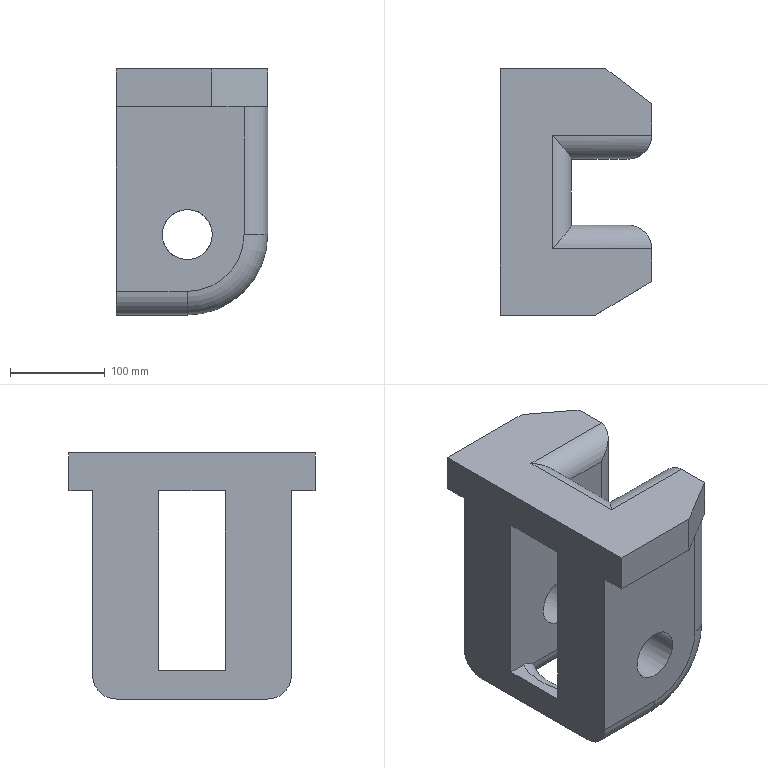Part | NX | features solid 2 | 1 solid | 37 faces | box 160 x 260 x 260 mm | volume 5588314 mm3 | plane 17 | cylinder 15 | torus 5 | commonest cylinder face diameters 50 x10 53 x2 170 x2 40 x1
STEP:
#1=CARTESIAN_POINT('',(710.,440.,280.));
#2=VERTEX_POINT('',#1);
#3=CARTESIAN_POINT('',(765.,440.,280.));
#4=VERTEX_POINT('',#3);
#5=CARTESIAN_POINT('',(710.,440.,280.));
#6=DIRECTION('',(1.,0.,0.));
#7=VECTOR('',#6,1000.);
#8=LINE('',#5,#7);
#9=EDGE_CURVE('',#2,#4,#8,.T.);
#10=ORIENTED_EDGE('',*,*,#9,.T.);
#11=CARTESIAN_POINT('',(784.365,440.,295.));
#12=VERTEX_POINT('',#11);
#13=CARTESIAN_POINT('',(765.,440.,300.));
#14=DIRECTION('',(0.,1.,0.));
#15=DIRECTION('',(0.,0.,-1.));
#16=AXIS2_PLACEMENT_3D('',#13,#14,#15);
#17=CIRCLE('',#16,20.);
#18=EDGE_CURVE('',#4,#12,#17,.F.);
#19=ORIENTED_EDGE('',*,*,#18,.T.);
#20=CARTESIAN_POINT('',(845.,440.,295.));
#21=VERTEX_POINT('',#20);
#22=CARTESIAN_POINT('',(710.,440.,295.));
#23=DIRECTION('',(1.,0.,0.));
#24=VECTOR('',#23,1000.);
#25=LINE('',#22,#24);
#26=EDGE_CURVE('',#21,#12,#25,.F.);
#27=ORIENTED_EDGE('',*,*,#26,.F.);
#28=CARTESIAN_POINT('',(845.,440.,145.));
#29=VERTEX_POINT('',#28);
#30=CARTESIAN_POINT('',(845.,440.,35.));
#31=DIRECTION('',(0.,0.,-1.));
#32=VECTOR('',#31,1000.);
#33=LINE('',#30,#32);
#34=EDGE_CURVE('',#29,#21,#33,.F.);
#35=ORIENTED_EDGE('',*,*,#34,.F.);
#36=CARTESIAN_POINT('',(785.,440.,85.));
#37=VERTEX_POINT('',#36);
#38=CARTESIAN_POINT('',(785.,440.,145.));
#39=DIRECTION('',(0.,-1.,0.));
#40=DIRECTION('',(0.,0.,1.));
#41=AXIS2_PLACEMENT_3D('',#38,#39,#40);
#42=CIRCLE('',#41,60.);
#43=EDGE_CURVE('',#37,#29,#42,.T.);
#44=ORIENTED_EDGE('',*,*,#43,.F.);
#45=CARTESIAN_POINT('',(741.634,440.,85.));
#46=VERTEX_POINT('',#45);
#47=CARTESIAN_POINT('',(710.,440.,85.));
#48=DIRECTION('',(-1.,0.,0.));
#49=VECTOR('',#48,1000.);
#50=LINE('',#47,#49);
#51=EDGE_CURVE('',#46,#37,#50,.F.);
#52=ORIENTED_EDGE('',*,*,#51,.F.);
#53=CARTESIAN_POINT('',(728.668,440.,90.));
#54=VERTEX_POINT('',#53);
#55=CARTESIAN_POINT('',(728.668,440.,90.));
#56=CARTESIAN_POINT('',(733.411,440.,90.));
#57=CARTESIAN_POINT('',(738.187,440.,88.222));
#58=CARTESIAN_POINT('',(741.634,440.,85.));
#59=B_SPLINE_CURVE_WITH_KNOTS('',3,(#55,#56,#57,#58),.UNSPECIFIED.,.F.,.F.,(4,4),(0.08783,0.102),.UNSPECIFIED.);
#60=EDGE_CURVE('',#54,#46,#59,.T.);
#61=ORIENTED_EDGE('',*,*,#60,.F.);
#62=CARTESIAN_POINT('',(710.,440.,90.));
#63=VERTEX_POINT('',#62);
#64=CARTESIAN_POINT('',(710.,440.,90.));
#65=DIRECTION('',(-1.,0.,0.));
#66=VECTOR('',#65,1000.);
#67=LINE('',#64,#66);
#68=EDGE_CURVE('',#54,#63,#67,.T.);
#69=ORIENTED_EDGE('',*,*,#68,.T.);
#70=CARTESIAN_POINT('',(710.,440.,270.));
#71=DIRECTION('',(0.,0.,-1.));
#72=VECTOR('',#71,1000.);
#73=LINE('',#70,#72);
#74=EDGE_CURVE('',#2,#63,#73,.T.);
#75=ORIENTED_EDGE('',*,*,#74,.F.);
#76=EDGE_LOOP('',(#10,#19,#27,#35,#44,#52,#61,#69,#75));
#77=FACE_BOUND('',#76,.T.);
#78=CARTESIAN_POINT('',(785.,440.,171.5));
#79=VERTEX_POINT('',#78);
#80=CARTESIAN_POINT('',(785.,440.,145.));
#81=DIRECTION('',(0.,-1.,0.));
#82=DIRECTION('',(0.,0.,1.));
#83=AXIS2_PLACEMENT_3D('',#80,#81,#82);
#84=CIRCLE('',#83,26.5);
#85=EDGE_CURVE('',#79,#79,#84,.F.);
#86=ORIENTED_EDGE('',*,*,#85,.F.);
#87=EDGE_LOOP('',(#86));
#88=FACE_BOUND('',#87,.T.);
#89=CARTESIAN_POINT('',(710.,440.,35.));
#90=DIRECTION('',(0.,1.,0.));
#91=DIRECTION('',(0.,0.,1.));
#92=AXIS2_PLACEMENT_3D('',#89,#90,#91);
#93=PLANE('',#92);
#94=ADVANCED_FACE('',(#77,#88),#93,.T.);
#95=CARTESIAN_POINT('',(750.,535.,60.));
#96=VERTEX_POINT('',#95);
#97=CARTESIAN_POINT('',(750.,415.,60.));
#98=VERTEX_POINT('',#97);
#99=CARTESIAN_POINT('',(795.,475.,60.));
#100=DIRECTION('',(0.,0.,-1.));
#101=DIRECTION('',(0.,-1.,0.));
#102=AXIS2_PLACEMENT_3D('',#99,#100,#101);
#103=CIRCLE('',#102,75.);
#104=EDGE_CURVE('',#96,#98,#103,.F.);
#105=ORIENTED_EDGE('',*,*,#104,.F.);
#106=CARTESIAN_POINT('',(741.634,510.,85.));
#107=VERTEX_POINT('',#106);
#108=CARTESIAN_POINT('',(750.,535.,60.));
#109=CARTESIAN_POINT('',(749.855,531.571,60.));
#110=CARTESIAN_POINT('',(749.883,524.653,61.451));
#111=CARTESIAN_POINT('',(749.735,516.09,67.563));
#112=CARTESIAN_POINT('',(747.852,510.77,76.551));
#113=CARTESIAN_POINT('',(744.179,510.,82.62));
#114=CARTESIAN_POINT('',(741.634,510.,85.));
#115=B_SPLINE_CURVE_WITH_KNOTS('',3,(#108,#109,#110,#111,#112,#113,#114),.UNSPECIFIED.,.F.,.F.,(4,1,1,1,4),(-0.00004428,0.01025,0.02055,0.03084,0.04114),.UNSPECIFIED.);
#116=EDGE_CURVE('',#96,#107,#115,.T.);
#117=ORIENTED_EDGE('',*,*,#116,.T.);
#118=CARTESIAN_POINT('',(728.668,510.,90.));
#119=VERTEX_POINT('',#118);
#120=CARTESIAN_POINT('',(741.634,510.,85.));
#121=CARTESIAN_POINT('',(738.185,510.,88.224));
#122=CARTESIAN_POINT('',(733.403,510.,90.));
#123=CARTESIAN_POINT('',(728.668,510.,90.));
#124=B_SPLINE_CURVE_WITH_KNOTS('',3,(#120,#121,#122,#123),.UNSPECIFIED.,.F.,.F.,(4,4),(0.0024,0.01656),.UNSPECIFIED.);
#125=EDGE_CURVE('',#107,#119,#124,.T.);
#126=ORIENTED_EDGE('',*,*,#125,.T.);
#127=CARTESIAN_POINT('',(795.,475.,90.));
#128=DIRECTION('',(0.,0.,-1.));
#129=DIRECTION('',(0.,-1.,0.));
#130=AXIS2_PLACEMENT_3D('',#127,#128,#129);
#131=CIRCLE('',#130,75.);
#132=EDGE_CURVE('',#54,#119,#131,.T.);
#133=ORIENTED_EDGE('',*,*,#132,.F.);
#134=ORIENTED_EDGE('',*,*,#60,.T.);
#135=CARTESIAN_POINT('',(741.634,440.,85.));
#136=CARTESIAN_POINT('',(744.172,440.,82.627));
#137=CARTESIAN_POINT('',(747.832,439.25,76.604));
#138=CARTESIAN_POINT('',(749.739,433.909,67.556));
#139=CARTESIAN_POINT('',(749.882,425.357,61.456));
#140=CARTESIAN_POINT('',(749.856,418.421,60.));
#141=CARTESIAN_POINT('',(750.,415.,60.));
#142=B_SPLINE_CURVE_WITH_KNOTS('',3,(#135,#136,#137,#138,#139,#140,#141),.UNSPECIFIED.,.F.,.F.,(4,1,1,1,4),(0.000000289,0.01027,0.02055,0.03082,0.04109),.UNSPECIFIED.);
#143=EDGE_CURVE('',#46,#98,#142,.T.);
#144=ORIENTED_EDGE('',*,*,#143,.T.);
#145=EDGE_LOOP('',(#105,#117,#126,#133,#134,#144));
#146=FACE_BOUND('',#145,.T.);
#147=CARTESIAN_POINT('',(795.,475.,75.));
#148=DIRECTION('',(0.,0.,-1.));
#149=DIRECTION('',(0.,-1.,0.));
#150=AXIS2_PLACEMENT_3D('',#147,#148,#149);
#151=TOROIDAL_SURFACE('',#150,75.,15.);
#152=ADVANCED_FACE('',(#146),#151,.T.);
#153=CARTESIAN_POINT('',(710.,555.,60.));
#154=VERTEX_POINT('',#153);
#155=CARTESIAN_POINT('',(710.,395.,60.));
#156=VERTEX_POINT('',#155);
#157=CARTESIAN_POINT('',(710.,455.,60.));
#158=DIRECTION('',(0.,-1.,0.));
#159=VECTOR('',#158,1000.);
#160=LINE('',#157,#159);
#161=EDGE_CURVE('',#154,#156,#160,.T.);
#162=ORIENTED_EDGE('',*,*,#161,.F.);
#163=CARTESIAN_POINT('',(785.,555.,60.));
#164=VERTEX_POINT('',#163);
#165=CARTESIAN_POINT('',(785.,555.,60.));
#166=DIRECTION('',(1.,0.,0.));
#167=VECTOR('',#166,1000.);
#168=LINE('',#165,#167);
#169=EDGE_CURVE('',#164,#154,#168,.F.);
#170=ORIENTED_EDGE('',*,*,#169,.F.);
#171=CARTESIAN_POINT('',(785.,535.,60.));
#172=VERTEX_POINT('',#171);
#173=CARTESIAN_POINT('',(785.,455.,60.));
#174=DIRECTION('',(0.,1.,0.));
#175=VECTOR('',#174,1000.);
#176=LINE('',#173,#175);
#177=EDGE_CURVE('',#172,#164,#176,.T.);
#178=ORIENTED_EDGE('',*,*,#177,.F.);
#179=CARTESIAN_POINT('',(785.,535.,60.));
#180=DIRECTION('',(-1.,0.,0.));
#181=VECTOR('',#180,1000.);
#182=LINE('',#179,#181);
#183=EDGE_CURVE('',#96,#172,#182,.F.);
#184=ORIENTED_EDGE('',*,*,#183,.F.);
#185=ORIENTED_EDGE('',*,*,#104,.T.);
#186=CARTESIAN_POINT('',(785.,415.,60.));
#187=VERTEX_POINT('',#186);
#188=CARTESIAN_POINT('',(785.,415.,60.));
#189=DIRECTION('',(-1.,0.,0.));
#190=VECTOR('',#189,1000.);
#191=LINE('',#188,#190);
#192=EDGE_CURVE('',#187,#98,#191,.T.);
#193=ORIENTED_EDGE('',*,*,#192,.F.);
#194=CARTESIAN_POINT('',(785.,395.,60.));
#195=VERTEX_POINT('',#194);
#196=CARTESIAN_POINT('',(785.,315.,60.));
#197=DIRECTION('',(0.,1.,0.));
#198=VECTOR('',#197,1000.);
#199=LINE('',#196,#198);
#200=EDGE_CURVE('',#195,#187,#199,.T.);
#201=ORIENTED_EDGE('',*,*,#200,.F.);
#202=CARTESIAN_POINT('',(785.,395.,60.));
#203=DIRECTION('',(1.,0.,0.));
#204=VECTOR('',#203,1000.);
#205=LINE('',#202,#204);
#206=EDGE_CURVE('',#156,#195,#205,.T.);
#207=ORIENTED_EDGE('',*,*,#206,.F.);
#208=EDGE_LOOP('',(#162,#170,#178,#184,#185,#193,#201,#207));
#209=FACE_BOUND('',#208,.T.);
#210=CARTESIAN_POINT('',(785.,455.,60.));
#211=DIRECTION('',(0.,0.,-1.));
#212=DIRECTION('',(-1.,0.,0.));
#213=AXIS2_PLACEMENT_3D('',#210,#211,#212);
#214=PLANE('',#213);
#215=ADVANCED_FACE('',(#209),#214,.T.);
#216=CARTESIAN_POINT('',(765.,415.,320.));
#217=VERTEX_POINT('',#216);
#218=CARTESIAN_POINT('',(784.365,440.,295.));
#219=CARTESIAN_POINT('',(784.836,440.,296.824));
#220=CARTESIAN_POINT('',(785.148,439.689,299.624));
#221=CARTESIAN_POINT('',(784.832,438.765,302.842));
#222=CARTESIAN_POINT('',(784.481,438.097,304.604));
#223=CARTESIAN_POINT('',(784.097,437.471,305.986));
#224=CARTESIAN_POINT('',(783.748,436.945,306.992));
#225=CARTESIAN_POINT('',(783.16,436.104,308.447));
#226=CARTESIAN_POINT('',(782.267,434.912,310.182));
#227=CARTESIAN_POINT('',(781.153,433.51,311.844));
#228=CARTESIAN_POINT('',(780.247,432.405,312.954));
#229=CARTESIAN_POINT('',(779.714,431.764,313.551));
#230=CARTESIAN_POINT('',(779.249,431.207,314.038));
#231=CARTESIAN_POINT('',(778.959,430.862,314.325));
#232=CARTESIAN_POINT('',(778.49,430.306,314.772));
#233=CARTESIAN_POINT('',(777.656,429.324,315.509));
#234=CARTESIAN_POINT('',(776.589,428.081,316.326));
#235=CARTESIAN_POINT('',(775.424,426.742,317.08));
#236=CARTESIAN_POINT('',(774.497,425.682,317.612));
#237=CARTESIAN_POINT('',(773.688,424.763,318.021));
#238=CARTESIAN_POINT('',(773.089,424.083,318.293));
#239=CARTESIAN_POINT('',(772.758,423.709,318.435));
#240=CARTESIAN_POINT('',(772.456,423.367,318.559));
#241=CARTESIAN_POINT('',(772.346,423.243,318.602));
#242=CARTESIAN_POINT('',(772.124,422.991,318.689));
#243=CARTESIAN_POINT('',(771.748,422.566,318.83));
#244=CARTESIAN_POINT('',(771.144,421.881,319.039));
#245=CARTESIAN_POINT('',(770.34,420.973,319.281));
#246=CARTESIAN_POINT('',(769.15,419.635,319.582));
#247=CARTESIAN_POINT('',(767.445,417.727,319.892));
#248=CARTESIAN_POINT('',(765.851,415.951,320.));
#249=CARTESIAN_POINT('',(765.,415.,320.));
#250=B_SPLINE_CURVE_WITH_KNOTS('',3,(#218,#219,#220,#221,#222,#223,#224,#225,#226,#227,#228,#229,#230,#231,#232,#233,#234,#235,#236,#237,#238,#239,#240,#241,#242,#243,#244,#245,#246,#247,#248,#249),.UNSPECIFIED.,.F.,.F.,(4,1,1,1,1,1,1,1,1,1,1,1,1,1,1,1,1,1,1,1,1,1,1,1,1,1,1,1,1,4),(0.,0.125,0.1875,0.2188,0.25,0.2812,0.3125,0.375,0.4375,0.4688,0.4844,0.5,0.5156,0.5312,0.5625,0.625,0.6562,0.6875,0.7188,0.7344,0.7422,0.75,0.7578,0.7656,0.7812,0.8125,0.8438,0.875,0.9375,1.),.UNSPECIFIED.);
#251=EDGE_CURVE('',#12,#217,#250,.T.);
#252=ORIENTED_EDGE('',*,*,#251,.F.);
#253=ORIENTED_EDGE('',*,*,#18,.F.);
#254=CARTESIAN_POINT('',(765.,510.,280.));
#255=VERTEX_POINT('',#254);
#256=CARTESIAN_POINT('',(765.,400.,280.));
#257=DIRECTION('',(0.,1.,0.));
#258=VECTOR('',#257,1000.);
#259=LINE('',#256,#258);
#260=EDGE_CURVE('',#255,#4,#259,.F.);
#261=ORIENTED_EDGE('',*,*,#260,.F.);
#262=CARTESIAN_POINT('',(784.365,510.,295.));
#263=VERTEX_POINT('',#262);
#264=CARTESIAN_POINT('',(765.,510.,300.));
#265=DIRECTION('',(0.,1.,0.));
#266=DIRECTION('',(0.,0.,-1.));
#267=AXIS2_PLACEMENT_3D('',#264,#265,#266);
#268=CIRCLE('',#267,20.);
#269=EDGE_CURVE('',#263,#255,#268,.T.);
#270=ORIENTED_EDGE('',*,*,#269,.F.);
#271=CARTESIAN_POINT('',(765.,535.,320.));
#272=VERTEX_POINT('',#271);
#273=CARTESIAN_POINT('',(784.365,510.,295.));
#274=CARTESIAN_POINT('',(784.836,510.,296.824));
#275=CARTESIAN_POINT('',(785.148,510.311,299.624));
#276=CARTESIAN_POINT('',(784.832,511.235,302.842));
#277=CARTESIAN_POINT('',(784.481,511.903,304.604));
#278=CARTESIAN_POINT('',(784.097,512.529,305.986));
#279=CARTESIAN_POINT('',(783.748,513.055,306.992));
#280=CARTESIAN_POINT('',(783.16,513.896,308.447));
#281=CARTESIAN_POINT('',(782.267,515.088,310.182));
#282=CARTESIAN_POINT('',(781.153,516.49,311.844));
#283=CARTESIAN_POINT('',(780.247,517.595,312.954));
#284=CARTESIAN_POINT('',(779.714,518.236,313.551));
#285=CARTESIAN_POINT('',(779.249,518.793,314.038));
#286=CARTESIAN_POINT('',(778.959,519.138,314.325));
#287=CARTESIAN_POINT('',(778.49,519.694,314.772));
#288=CARTESIAN_POINT('',(777.656,520.676,315.509));
#289=CARTESIAN_POINT('',(776.589,521.919,316.326));
#290=CARTESIAN_POINT('',(775.424,523.258,317.08));
#291=CARTESIAN_POINT('',(774.497,524.318,317.612));
#292=CARTESIAN_POINT('',(773.688,525.237,318.021));
#293=CARTESIAN_POINT('',(773.089,525.917,318.293));
#294=CARTESIAN_POINT('',(772.758,526.291,318.435));
#295=CARTESIAN_POINT('',(772.456,526.633,318.559));
#296=CARTESIAN_POINT('',(772.346,526.757,318.602));
#297=CARTESIAN_POINT('',(772.124,527.009,318.689));
#298=CARTESIAN_POINT('',(771.748,527.434,318.83));
#299=CARTESIAN_POINT('',(771.144,528.119,319.039));
#300=CARTESIAN_POINT('',(770.34,529.027,319.281));
#301=CARTESIAN_POINT('',(769.15,530.365,319.582));
#302=CARTESIAN_POINT('',(767.445,532.273,319.892));
#303=CARTESIAN_POINT('',(765.851,534.049,320.));
#304=CARTESIAN_POINT('',(765.,535.,320.));
#305=B_SPLINE_CURVE_WITH_KNOTS('',3,(#273,#274,#275,#276,#277,#278,#279,#280,#281,#282,#283,#284,#285,#286,#287,#288,#289,#290,#291,#292,#293,#294,#295,#296,#297,#298,#299,#300,#301,#302,#303,#304),.UNSPECIFIED.,.F.,.F.,(4,1,1,1,1,1,1,1,1,1,1,1,1,1,1,1,1,1,1,1,1,1,1,1,1,1,1,1,1,4),(0.,0.125,0.1875,0.2188,0.25,0.2812,0.3125,0.375,0.4375,0.4688,0.4844,0.5,0.5156,0.5312,0.5625,0.625,0.6562,0.6875,0.7188,0.7344,0.7422,0.75,0.7578,0.7656,0.7812,0.8125,0.8438,0.875,0.9375,1.),.UNSPECIFIED.);
#306=EDGE_CURVE('',#263,#272,#305,.T.);
#307=ORIENTED_EDGE('',*,*,#306,.T.);
#308=CARTESIAN_POINT('',(765.,510.,320.));
#309=DIRECTION('',(0.,1.,0.));
#310=VECTOR('',#309,1000.);
#311=LINE('',#308,#310);
#312=EDGE_CURVE('',#217,#272,#311,.T.);
#313=ORIENTED_EDGE('',*,*,#312,.F.);
#314=EDGE_LOOP('',(#252,#253,#261,#270,#307,#313));
#315=FACE_BOUND('',#314,.T.);
#316=CARTESIAN_POINT('',(765.,510.,300.));
#317=DIRECTION('',(0.,-1.,0.));
#318=DIRECTION('',(0.,0.,1.));
#319=AXIS2_PLACEMENT_3D('',#316,#317,#318);
#320=CYLINDRICAL_SURFACE('',#319,20.);
#321=ADVANCED_FACE('',(#315),#320,.T.);
#322=ORIENTED_EDGE('',*,*,#312,.T.);
#323=CARTESIAN_POINT('',(870.,535.,320.));
#324=VERTEX_POINT('',#323);
#325=CARTESIAN_POINT('',(765.,535.,320.));
#326=DIRECTION('',(1.,0.,0.));
#327=VECTOR('',#326,1000.);
#328=LINE('',#325,#327);
#329=EDGE_CURVE('',#324,#272,#328,.F.);
#330=ORIENTED_EDGE('',*,*,#329,.F.);
#331=CARTESIAN_POINT('',(870.,568.232,320.));
#332=VERTEX_POINT('',#331);
#333=CARTESIAN_POINT('',(870.,455.,320.));
#334=DIRECTION('',(0.,-1.,0.));
#335=VECTOR('',#334,1000.);
#336=LINE('',#333,#335);
#337=EDGE_CURVE('',#332,#324,#336,.T.);
#338=ORIENTED_EDGE('',*,*,#337,.F.);
#339=CARTESIAN_POINT('',(821.621,605.,320.));
#340=VERTEX_POINT('',#339);
#341=CARTESIAN_POINT('',(938.114,516.465,320.));
#342=DIRECTION('',(0.7962,-0.6051,0.));
#343=VECTOR('',#342,1000.);
#344=LINE('',#341,#343);
#345=EDGE_CURVE('',#332,#340,#344,.F.);
#346=ORIENTED_EDGE('',*,*,#345,.T.);
#347=CARTESIAN_POINT('',(710.,605.,320.));
#348=VERTEX_POINT('',#347);
#349=CARTESIAN_POINT('',(10.,605.,320.));
#350=DIRECTION('',(1.,0.,0.));
#351=VECTOR('',#350,1000.);
#352=LINE('',#349,#351);
#353=EDGE_CURVE('',#340,#348,#352,.F.);
#354=ORIENTED_EDGE('',*,*,#353,.T.);
#355=CARTESIAN_POINT('',(710.,345.,320.));
#356=VERTEX_POINT('',#355);
#357=CARTESIAN_POINT('',(710.,510.,320.));
#358=DIRECTION('',(0.,1.,0.));
#359=VECTOR('',#358,1000.);
#360=LINE('',#357,#359);
#361=EDGE_CURVE('',#348,#356,#360,.F.);
#362=ORIENTED_EDGE('',*,*,#361,.T.);
#363=CARTESIAN_POINT('',(810.84,345.,320.));
#364=VERTEX_POINT('',#363);
#365=CARTESIAN_POINT('',(785.,345.,320.));
#366=DIRECTION('',(-1.,0.,0.));
#367=VECTOR('',#366,1000.);
#368=LINE('',#365,#367);
#369=EDGE_CURVE('',#364,#356,#368,.T.);
#370=ORIENTED_EDGE('',*,*,#369,.F.);
#371=CARTESIAN_POINT('',(870.,380.496,320.));
#372=VERTEX_POINT('',#371);
#373=CARTESIAN_POINT('',(778.605,325.659,320.));
#374=DIRECTION('',(0.8575,0.5145,0.));
#375=VECTOR('',#374,1000.);
#376=LINE('',#373,#375);
#377=EDGE_CURVE('',#364,#372,#376,.T.);
#378=ORIENTED_EDGE('',*,*,#377,.T.);
#379=CARTESIAN_POINT('',(870.,415.,320.));
#380=VERTEX_POINT('',#379);
#381=CARTESIAN_POINT('',(870.,315.,320.));
#382=DIRECTION('',(0.,-1.,0.));
#383=VECTOR('',#382,1000.);
#384=LINE('',#381,#383);
#385=EDGE_CURVE('',#380,#372,#384,.T.);
#386=ORIENTED_EDGE('',*,*,#385,.F.);
#387=CARTESIAN_POINT('',(785.,415.,320.));
#388=DIRECTION('',(1.,0.,0.));
#389=VECTOR('',#388,1000.);
#390=LINE('',#387,#389);
#391=EDGE_CURVE('',#217,#380,#390,.T.);
#392=ORIENTED_EDGE('',*,*,#391,.F.);
#393=EDGE_LOOP('',(#322,#330,#338,#346,#354,#362,#370,#378,#386,#392));
#394=FACE_BOUND('',#393,.T.);
#395=CARTESIAN_POINT('',(710.,510.,320.));
#396=DIRECTION('',(0.,0.,-1.));
#397=DIRECTION('',(0.,1.,0.));
#398=AXIS2_PLACEMENT_3D('',#395,#396,#397);
#399=PLANE('',#398);
#400=ADVANCED_FACE('',(#394),#399,.F.);
#401=CARTESIAN_POINT('',(710.,510.,90.));
#402=VERTEX_POINT('',#401);
#403=CARTESIAN_POINT('',(710.,510.,280.));
#404=VERTEX_POINT('',#403);
#405=CARTESIAN_POINT('',(710.,510.,60.));
#406=DIRECTION('',(0.,0.,1.));
#407=VECTOR('',#406,1000.);
#408=LINE('',#405,#407);
#409=EDGE_CURVE('',#402,#404,#408,.T.);
#410=ORIENTED_EDGE('',*,*,#409,.T.);
#411=CARTESIAN_POINT('',(710.,510.,280.));
#412=DIRECTION('',(0.,1.,0.));
#413=VECTOR('',#412,1000.);
#414=LINE('',#411,#413);
#415=EDGE_CURVE('',#404,#2,#414,.F.);
#416=ORIENTED_EDGE('',*,*,#415,.T.);
#417=ORIENTED_EDGE('',*,*,#74,.T.);
#418=CARTESIAN_POINT('',(710.,510.,90.));
#419=DIRECTION('',(0.,-1.,0.));
#420=VECTOR('',#419,1000.);
#421=LINE('',#418,#420);
#422=EDGE_CURVE('',#402,#63,#421,.T.);
#423=ORIENTED_EDGE('',*,*,#422,.F.);
#424=EDGE_LOOP('',(#410,#416,#417,#423));
#425=FACE_BOUND('',#424,.T.);
#426=ORIENTED_EDGE('',*,*,#361,.F.);
#427=CARTESIAN_POINT('',(710.,605.,280.));
#428=VERTEX_POINT('',#427);
#429=CARTESIAN_POINT('',(710.,605.,155.));
#430=DIRECTION('',(0.,0.,1.));
#431=VECTOR('',#430,1000.);
#432=LINE('',#429,#431);
#433=EDGE_CURVE('',#348,#428,#432,.F.);
#434=ORIENTED_EDGE('',*,*,#433,.T.);
#435=CARTESIAN_POINT('',(710.,580.,280.));
#436=VERTEX_POINT('',#435);
#437=CARTESIAN_POINT('',(710.,620.,280.));
#438=DIRECTION('',(0.,-1.,0.));
#439=VECTOR('',#438,1000.);
#440=LINE('',#437,#439);
#441=EDGE_CURVE('',#428,#436,#440,.T.);
#442=ORIENTED_EDGE('',*,*,#441,.T.);
#443=CARTESIAN_POINT('',(710.,580.,85.));
#444=VERTEX_POINT('',#443);
#445=CARTESIAN_POINT('',(710.,580.,95.));
#446=DIRECTION('',(0.,0.,-1.));
#447=VECTOR('',#446,1000.);
#448=LINE('',#445,#447);
#449=EDGE_CURVE('',#436,#444,#448,.T.);
#450=ORIENTED_EDGE('',*,*,#449,.T.);
#451=CARTESIAN_POINT('',(710.,555.,85.));
#452=DIRECTION('',(1.,0.,0.));
#453=DIRECTION('',(0.,0.,-1.));
#454=AXIS2_PLACEMENT_3D('',#451,#452,#453);
#455=CIRCLE('',#454,25.);
#456=EDGE_CURVE('',#154,#444,#455,.T.);
#457=ORIENTED_EDGE('',*,*,#456,.F.);
#458=ORIENTED_EDGE('',*,*,#161,.T.);
#459=CARTESIAN_POINT('',(710.,370.,85.));
#460=VERTEX_POINT('',#459);
#461=CARTESIAN_POINT('',(710.,395.,85.));
#462=DIRECTION('',(1.,0.,0.));
#463=DIRECTION('',(0.,0.,-1.));
#464=AXIS2_PLACEMENT_3D('',#461,#462,#463);
#465=CIRCLE('',#464,25.);
#466=EDGE_CURVE('',#460,#156,#465,.T.);
#467=ORIENTED_EDGE('',*,*,#466,.F.);
#468=CARTESIAN_POINT('',(710.,370.,280.));
#469=VERTEX_POINT('',#468);
#470=CARTESIAN_POINT('',(710.,370.,70.));
#471=DIRECTION('',(0.,0.,1.));
#472=VECTOR('',#471,1000.);
#473=LINE('',#470,#472);
#474=EDGE_CURVE('',#460,#469,#473,.T.);
#475=ORIENTED_EDGE('',*,*,#474,.T.);
#476=CARTESIAN_POINT('',(710.,345.,280.));
#477=VERTEX_POINT('',#476);
#478=CARTESIAN_POINT('',(710.,285.,280.));
#479=DIRECTION('',(0.,-1.,0.));
#480=VECTOR('',#479,1000.);
#481=LINE('',#478,#480);
#482=EDGE_CURVE('',#469,#477,#481,.T.);
#483=ORIENTED_EDGE('',*,*,#482,.T.);
#484=CARTESIAN_POINT('',(710.,345.,245.));
#485=DIRECTION('',(0.,0.,-1.));
#486=VECTOR('',#485,1000.);
#487=LINE('',#484,#486);
#488=EDGE_CURVE('',#356,#477,#487,.T.);
#489=ORIENTED_EDGE('',*,*,#488,.F.);
#490=EDGE_LOOP('',(#426,#434,#442,#450,#457,#458,#467,#475,#483,#489));
#491=FACE_BOUND('',#490,.T.);
#492=CARTESIAN_POINT('',(710.,340.,270.));
#493=DIRECTION('',(-1.,0.,0.));
#494=DIRECTION('',(0.,-1.,0.));
#495=AXIS2_PLACEMENT_3D('',#492,#493,#494);
#496=PLANE('',#495);
#497=ADVANCED_FACE('',(#425,#491),#496,.T.);
#498=CARTESIAN_POINT('',(845.,370.,145.));
#499=VERTEX_POINT('',#498);
#500=CARTESIAN_POINT('',(870.,395.,145.));
#501=VERTEX_POINT('',#500);
#502=CARTESIAN_POINT('',(845.,395.,145.));
#503=DIRECTION('',(0.,0.,1.));
#504=DIRECTION('',(0.,1.,0.));
#505=AXIS2_PLACEMENT_3D('',#502,#503,#504);
#506=CIRCLE('',#505,25.);
#507=EDGE_CURVE('',#499,#501,#506,.T.);
#508=ORIENTED_EDGE('',*,*,#507,.F.);
#509=CARTESIAN_POINT('',(785.,370.,85.));
#510=VERTEX_POINT('',#509);
#511=CARTESIAN_POINT('',(785.,370.,145.));
#512=DIRECTION('',(0.,1.,0.));
#513=DIRECTION('',(0.,0.,-1.));
#514=AXIS2_PLACEMENT_3D('',#511,#512,#513);
#515=CIRCLE('',#514,60.);
#516=EDGE_CURVE('',#499,#510,#515,.T.);
#517=ORIENTED_EDGE('',*,*,#516,.T.);
#518=CARTESIAN_POINT('',(785.,395.,85.));
#519=DIRECTION('',(1.,0.,0.));
#520=DIRECTION('',(0.,0.,-1.));
#521=AXIS2_PLACEMENT_3D('',#518,#519,#520);
#522=CIRCLE('',#521,25.);
#523=EDGE_CURVE('',#510,#195,#522,.T.);
#524=ORIENTED_EDGE('',*,*,#523,.T.);
#525=CARTESIAN_POINT('',(785.,395.,145.));
#526=DIRECTION('',(0.,1.,0.));
#527=DIRECTION('',(0.,0.,-1.));
#528=AXIS2_PLACEMENT_3D('',#525,#526,#527);
#529=CIRCLE('',#528,85.);
#530=EDGE_CURVE('',#195,#501,#529,.F.);
#531=ORIENTED_EDGE('',*,*,#530,.T.);
#532=EDGE_LOOP('',(#508,#517,#524,#531));
#533=FACE_BOUND('',#532,.T.);
#534=CARTESIAN_POINT('',(785.,395.,145.));
#535=DIRECTION('',(0.,-1.,0.));
#536=DIRECTION('',(0.,0.,-1.));
#537=AXIS2_PLACEMENT_3D('',#534,#535,#536);
#538=TOROIDAL_SURFACE('',#537,60.,25.);
#539=ADVANCED_FACE('',(#533),#538,.T.);
#540=CARTESIAN_POINT('',(870.,395.,280.));
#541=VERTEX_POINT('',#540);
#542=CARTESIAN_POINT('',(870.,395.,70.));
#543=DIRECTION('',(0.,0.,-1.));
#544=VECTOR('',#543,1000.);
#545=LINE('',#542,#544);
#546=EDGE_CURVE('',#501,#541,#545,.F.);
#547=ORIENTED_EDGE('',*,*,#546,.T.);
#548=CARTESIAN_POINT('',(845.,370.,280.));
#549=VERTEX_POINT('',#548);
#550=CARTESIAN_POINT('',(845.,395.,280.));
#551=DIRECTION('',(0.,0.,1.));
#552=DIRECTION('',(0.,1.,0.));
#553=AXIS2_PLACEMENT_3D('',#550,#551,#552);
#554=CIRCLE('',#553,25.);
#555=EDGE_CURVE('',#541,#549,#554,.F.);
#556=ORIENTED_EDGE('',*,*,#555,.T.);
#557=CARTESIAN_POINT('',(845.,370.,70.));
#558=DIRECTION('',(0.,0.,-1.));
#559=VECTOR('',#558,1000.);
#560=LINE('',#557,#559);
#561=EDGE_CURVE('',#549,#499,#560,.T.);
#562=ORIENTED_EDGE('',*,*,#561,.T.);
#563=ORIENTED_EDGE('',*,*,#507,.T.);
#564=EDGE_LOOP('',(#547,#556,#562,#563));
#565=FACE_BOUND('',#564,.T.);
#566=CARTESIAN_POINT('',(845.,395.,70.));
#567=DIRECTION('',(0.,0.,-1.));
#568=DIRECTION('',(0.,1.,0.));
#569=AXIS2_PLACEMENT_3D('',#566,#567,#568);
#570=CYLINDRICAL_SURFACE('',#569,25.);
#571=ADVANCED_FACE('',(#565),#570,.T.);
#572=CARTESIAN_POINT('',(870.,415.,145.));
#573=VERTEX_POINT('',#572);
#574=CARTESIAN_POINT('',(845.,415.,145.));
#575=DIRECTION('',(0.,0.,1.));
#576=DIRECTION('',(0.,1.,0.));
#577=AXIS2_PLACEMENT_3D('',#574,#575,#576);
#578=CIRCLE('',#577,25.);
#579=EDGE_CURVE('',#573,#29,#578,.T.);
#580=ORIENTED_EDGE('',*,*,#579,.F.);
#581=CARTESIAN_POINT('',(785.,415.,145.));
#582=DIRECTION('',(0.,-1.,0.));
#583=DIRECTION('',(0.,0.,1.));
#584=AXIS2_PLACEMENT_3D('',#581,#582,#583);
#585=CIRCLE('',#584,85.);
#586=EDGE_CURVE('',#573,#187,#585,.F.);
#587=ORIENTED_EDGE('',*,*,#586,.T.);
#588=CARTESIAN_POINT('',(785.,415.,85.));
#589=DIRECTION('',(1.,0.,0.));
#590=DIRECTION('',(0.,0.,-1.));
#591=AXIS2_PLACEMENT_3D('',#588,#589,#590);
#592=CIRCLE('',#591,25.);
#593=EDGE_CURVE('',#187,#37,#592,.T.);
#594=ORIENTED_EDGE('',*,*,#593,.T.);
#595=ORIENTED_EDGE('',*,*,#43,.T.);
#596=EDGE_LOOP('',(#580,#587,#594,#595));
#597=FACE_BOUND('',#596,.T.);
#598=CARTESIAN_POINT('',(785.,415.,145.));
#599=DIRECTION('',(0.,1.,0.));
#600=DIRECTION('',(0.,0.,1.));
#601=AXIS2_PLACEMENT_3D('',#598,#599,#600);
#602=TOROIDAL_SURFACE('',#601,60.,25.);
#603=ADVANCED_FACE('',(#597),#602,.T.);
#604=ORIENTED_EDGE('',*,*,#34,.T.);
#605=CARTESIAN_POINT('',(845.,415.,295.));
#606=DIRECTION('',(-0.7071,0.,0.7071));
#607=DIRECTION('',(0.7071,0.,0.7071));
#608=AXIS2_PLACEMENT_3D('',#605,#606,#607);
#609=ELLIPSE('',#608,35.355,25.);
#610=EDGE_CURVE('',#380,#21,#609,.T.);
#611=ORIENTED_EDGE('',*,*,#610,.F.);
#612=CARTESIAN_POINT('',(870.,415.,70.));
#613=DIRECTION('',(0.,0.,-1.));
#614=VECTOR('',#613,1000.);
#615=LINE('',#612,#614);
#616=EDGE_CURVE('',#380,#573,#615,.T.);
#617=ORIENTED_EDGE('',*,*,#616,.T.);
#618=ORIENTED_EDGE('',*,*,#579,.T.);
#619=EDGE_LOOP('',(#604,#611,#617,#618));
#620=FACE_BOUND('',#619,.T.);
#621=CARTESIAN_POINT('',(845.,415.,70.));
#622=DIRECTION('',(0.,0.,-1.));
#623=DIRECTION('',(0.,1.,0.));
#624=AXIS2_PLACEMENT_3D('',#621,#622,#623);
#625=CYLINDRICAL_SURFACE('',#624,25.);
#626=ADVANCED_FACE('',(#620),#625,.T.);
#627=CARTESIAN_POINT('',(811.5,370.,145.));
#628=VERTEX_POINT('',#627);
#629=CARTESIAN_POINT('',(785.,370.,145.));
#630=DIRECTION('',(0.,1.,0.));
#631=DIRECTION('',(1.,0.,0.));
#632=AXIS2_PLACEMENT_3D('',#629,#630,#631);
#633=CIRCLE('',#632,26.5);
#634=EDGE_CURVE('',#628,#628,#633,.T.);
#635=ORIENTED_EDGE('',*,*,#634,.F.);
#636=EDGE_LOOP('',(#635));
#637=FACE_BOUND('',#636,.T.);
#638=ORIENTED_EDGE('',*,*,#85,.T.);
#639=EDGE_LOOP('',(#638));
#640=FACE_BOUND('',#639,.T.);
#641=CARTESIAN_POINT('',(785.,185.,145.));
#642=DIRECTION('',(0.,1.,0.));
#643=DIRECTION('',(-1.,0.,0.));
#644=AXIS2_PLACEMENT_3D('',#641,#642,#643);
#645=CYLINDRICAL_SURFACE('',#644,26.5);
#646=ADVANCED_FACE('',(#637,#640),#645,.F.);
#647=ORIENTED_EDGE('',*,*,#482,.F.);
#648=CARTESIAN_POINT('',(870.,370.,280.));
#649=DIRECTION('',(-1.,0.,0.));
#650=VECTOR('',#649,1000.);
#651=LINE('',#648,#650);
#652=EDGE_CURVE('',#549,#469,#651,.T.);
#653=ORIENTED_EDGE('',*,*,#652,.F.);
#654=ORIENTED_EDGE('',*,*,#555,.F.);
#655=CARTESIAN_POINT('',(870.,380.496,280.));
#656=VERTEX_POINT('',#655);
#657=CARTESIAN_POINT('',(870.,370.,280.));
#658=DIRECTION('',(0.,-1.,0.));
#659=VECTOR('',#658,1000.);
#660=LINE('',#657,#659);
#661=EDGE_CURVE('',#541,#656,#660,.T.);
#662=ORIENTED_EDGE('',*,*,#661,.T.);
#663=CARTESIAN_POINT('',(810.84,345.,280.));
#664=VERTEX_POINT('',#663);
#665=CARTESIAN_POINT('',(865.37,377.717,280.));
#666=DIRECTION('',(-0.8575,-0.5145,0.));
#667=VECTOR('',#666,1000.);
#668=LINE('',#665,#667);
#669=EDGE_CURVE('',#656,#664,#668,.T.);
#670=ORIENTED_EDGE('',*,*,#669,.T.);
#671=CARTESIAN_POINT('',(700.,345.,280.));
#672=DIRECTION('',(1.,0.,0.));
#673=VECTOR('',#672,1000.);
#674=LINE('',#671,#673);
#675=EDGE_CURVE('',#477,#664,#674,.T.);
#676=ORIENTED_EDGE('',*,*,#675,.F.);
#677=EDGE_LOOP('',(#647,#653,#654,#662,#670,#676));
#678=FACE_BOUND('',#677,.T.);
#679=CARTESIAN_POINT('',(700.,285.,280.));
#680=DIRECTION('',(0.,0.,-1.));
#681=DIRECTION('',(0.,-1.,0.));
#682=AXIS2_PLACEMENT_3D('',#679,#680,#681);
#683=PLANE('',#682);
#684=ADVANCED_FACE('',(#678),#683,.T.);
#685=ORIENTED_EDGE('',*,*,#516,.F.);
#686=ORIENTED_EDGE('',*,*,#561,.F.);
#687=ORIENTED_EDGE('',*,*,#652,.T.);
#688=ORIENTED_EDGE('',*,*,#474,.F.);
#689=CARTESIAN_POINT('',(785.,370.,85.));
#690=DIRECTION('',(1.,0.,0.));
#691=VECTOR('',#690,1000.);
#692=LINE('',#689,#691);
#693=EDGE_CURVE('',#510,#460,#692,.F.);
#694=ORIENTED_EDGE('',*,*,#693,.F.);
#695=EDGE_LOOP('',(#685,#686,#687,#688,#694));
#696=FACE_BOUND('',#695,.T.);
#697=ORIENTED_EDGE('',*,*,#634,.T.);
#698=EDGE_LOOP('',(#697));
#699=FACE_BOUND('',#698,.T.);
#700=CARTESIAN_POINT('',(785.,370.,70.));
#701=DIRECTION('',(0.,-1.,0.));
#702=DIRECTION('',(1.,0.,0.));
#703=AXIS2_PLACEMENT_3D('',#700,#701,#702);
#704=PLANE('',#703);
#705=ADVANCED_FACE('',(#696,#699),#704,.T.);
#706=ORIENTED_EDGE('',*,*,#466,.T.);
#707=ORIENTED_EDGE('',*,*,#206,.T.);
#708=ORIENTED_EDGE('',*,*,#523,.F.);
#709=ORIENTED_EDGE('',*,*,#693,.T.);
#710=EDGE_LOOP('',(#706,#707,#708,#709));
#711=FACE_BOUND('',#710,.T.);
#712=CARTESIAN_POINT('',(785.,395.,85.));
#713=DIRECTION('',(1.,0.,0.));
#714=DIRECTION('',(0.,0.,1.));
#715=AXIS2_PLACEMENT_3D('',#712,#713,#714);
#716=CYLINDRICAL_SURFACE('',#715,25.);
#717=ADVANCED_FACE('',(#711),#716,.T.);
#718=ORIENTED_EDGE('',*,*,#200,.T.);
#719=ORIENTED_EDGE('',*,*,#586,.F.);
#720=CARTESIAN_POINT('',(870.,315.,145.));
#721=DIRECTION('',(0.,1.,0.));
#722=VECTOR('',#721,1000.);
#723=LINE('',#720,#722);
#724=EDGE_CURVE('',#573,#501,#723,.F.);
#725=ORIENTED_EDGE('',*,*,#724,.T.);
#726=ORIENTED_EDGE('',*,*,#530,.F.);
#727=EDGE_LOOP('',(#718,#719,#725,#726));
#728=FACE_BOUND('',#727,.T.);
#729=CARTESIAN_POINT('',(785.,315.,145.));
#730=DIRECTION('',(0.,1.,0.));
#731=DIRECTION('',(-1.,0.,0.));
#732=AXIS2_PLACEMENT_3D('',#729,#730,#731);
#733=CYLINDRICAL_SURFACE('',#732,85.);
#734=ADVANCED_FACE('',(#728),#733,.T.);
#735=ORIENTED_EDGE('',*,*,#724,.F.);
#736=ORIENTED_EDGE('',*,*,#616,.F.);
#737=ORIENTED_EDGE('',*,*,#385,.T.);
#738=CARTESIAN_POINT('',(870.,380.496,70.));
#739=DIRECTION('',(0.,0.,-1.));
#740=VECTOR('',#739,1000.);
#741=LINE('',#738,#740);
#742=EDGE_CURVE('',#372,#656,#741,.T.);
#743=ORIENTED_EDGE('',*,*,#742,.T.);
#744=ORIENTED_EDGE('',*,*,#661,.F.);
#745=ORIENTED_EDGE('',*,*,#546,.F.);
#746=EDGE_LOOP('',(#735,#736,#737,#743,#744,#745));
#747=FACE_BOUND('',#746,.T.);
#748=CARTESIAN_POINT('',(870.,315.,70.));
#749=DIRECTION('',(1.,0.,0.));
#750=DIRECTION('',(0.,1.,0.));
#751=AXIS2_PLACEMENT_3D('',#748,#749,#750);
#752=PLANE('',#751);
#753=ADVANCED_FACE('',(#747),#752,.T.);
#754=ORIENTED_EDGE('',*,*,#669,.F.);
#755=ORIENTED_EDGE('',*,*,#742,.F.);
#756=ORIENTED_EDGE('',*,*,#377,.F.);
#757=CARTESIAN_POINT('',(810.84,345.,70.));
#758=DIRECTION('',(0.,0.,1.));
#759=VECTOR('',#758,1000.);
#760=LINE('',#757,#759);
#761=EDGE_CURVE('',#664,#364,#760,.T.);
#762=ORIENTED_EDGE('',*,*,#761,.F.);
#763=EDGE_LOOP('',(#754,#755,#756,#762));
#764=FACE_BOUND('',#763,.T.);
#765=CARTESIAN_POINT('',(865.37,377.717,70.));
#766=DIRECTION('',(0.5145,-0.8575,0.));
#767=DIRECTION('',(0.8575,0.5145,0.));
#768=AXIS2_PLACEMENT_3D('',#765,#766,#767);
#769=PLANE('',#768);
#770=ADVANCED_FACE('',(#764),#769,.T.);
#771=ORIENTED_EDGE('',*,*,#369,.T.);
#772=ORIENTED_EDGE('',*,*,#488,.T.);
#773=ORIENTED_EDGE('',*,*,#675,.T.);
#774=ORIENTED_EDGE('',*,*,#761,.T.);
#775=EDGE_LOOP('',(#771,#772,#773,#774));
#776=FACE_BOUND('',#775,.T.);
#777=CARTESIAN_POINT('',(710.,345.,280.));
#778=DIRECTION('',(0.,-1.,0.));
#779=DIRECTION('',(1.,0.,0.));
#780=AXIS2_PLACEMENT_3D('',#777,#778,#779);
#781=PLANE('',#780);
#782=ADVANCED_FACE('',(#776),#781,.T.);
#783=ORIENTED_EDGE('',*,*,#26,.T.);
#784=ORIENTED_EDGE('',*,*,#251,.T.);
#785=ORIENTED_EDGE('',*,*,#391,.T.);
#786=ORIENTED_EDGE('',*,*,#610,.T.);
#787=EDGE_LOOP('',(#783,#784,#785,#786));
#788=FACE_BOUND('',#787,.T.);
#789=CARTESIAN_POINT('',(785.,415.,295.));
#790=DIRECTION('',(1.,0.,0.));
#791=DIRECTION('',(0.,0.,1.));
#792=AXIS2_PLACEMENT_3D('',#789,#790,#791);
#793=CYLINDRICAL_SURFACE('',#792,25.);
#794=ADVANCED_FACE('',(#788),#793,.T.);
#795=ORIENTED_EDGE('',*,*,#143,.F.);
#796=ORIENTED_EDGE('',*,*,#51,.T.);
#797=ORIENTED_EDGE('',*,*,#593,.F.);
#798=ORIENTED_EDGE('',*,*,#192,.T.);
#799=EDGE_LOOP('',(#795,#796,#797,#798));
#800=FACE_BOUND('',#799,.T.);
#801=CARTESIAN_POINT('',(785.,415.,85.));
#802=DIRECTION('',(-1.,0.,0.));
#803=DIRECTION('',(0.,0.,-1.));
#804=AXIS2_PLACEMENT_3D('',#801,#802,#803);
#805=CYLINDRICAL_SURFACE('',#804,25.);
#806=ADVANCED_FACE('',(#800),#805,.T.);
#807=ORIENTED_EDGE('',*,*,#132,.T.);
#808=CARTESIAN_POINT('',(710.,510.,90.));
#809=DIRECTION('',(1.,0.,0.));
#810=VECTOR('',#809,1000.);
#811=LINE('',#808,#810);
#812=EDGE_CURVE('',#402,#119,#811,.T.);
#813=ORIENTED_EDGE('',*,*,#812,.F.);
#814=ORIENTED_EDGE('',*,*,#422,.T.);
#815=ORIENTED_EDGE('',*,*,#68,.F.);
#816=EDGE_LOOP('',(#807,#813,#814,#815));
#817=FACE_BOUND('',#816,.T.);
#818=CARTESIAN_POINT('',(710.,510.,90.));
#819=DIRECTION('',(0.,0.,-1.));
#820=DIRECTION('',(0.,1.,0.));
#821=AXIS2_PLACEMENT_3D('',#818,#819,#820);
#822=PLANE('',#821);
#823=ADVANCED_FACE('',(#817),#822,.F.);
#824=ORIENTED_EDGE('',*,*,#269,.T.);
#825=CARTESIAN_POINT('',(710.,510.,280.));
#826=DIRECTION('',(-1.,0.,0.));
#827=VECTOR('',#826,1000.);
#828=LINE('',#825,#827);
#829=EDGE_CURVE('',#255,#404,#828,.T.);
#830=ORIENTED_EDGE('',*,*,#829,.T.);
#831=ORIENTED_EDGE('',*,*,#409,.F.);
#832=ORIENTED_EDGE('',*,*,#812,.T.);
#833=ORIENTED_EDGE('',*,*,#125,.F.);
#834=CARTESIAN_POINT('',(785.,510.,85.));
#835=VERTEX_POINT('',#834);
#836=CARTESIAN_POINT('',(710.,510.,85.));
#837=DIRECTION('',(-1.,0.,0.));
#838=VECTOR('',#837,1000.);
#839=LINE('',#836,#838);
#840=EDGE_CURVE('',#835,#107,#839,.T.);
#841=ORIENTED_EDGE('',*,*,#840,.F.);
#842=CARTESIAN_POINT('',(845.,510.,145.));
#843=VERTEX_POINT('',#842);
#844=CARTESIAN_POINT('',(785.,510.,145.));
#845=DIRECTION('',(0.,-1.,0.));
#846=DIRECTION('',(0.,0.,1.));
#847=AXIS2_PLACEMENT_3D('',#844,#845,#846);
#848=CIRCLE('',#847,60.);
#849=EDGE_CURVE('',#843,#835,#848,.F.);
#850=ORIENTED_EDGE('',*,*,#849,.F.);
#851=CARTESIAN_POINT('',(845.,510.,295.));
#852=VERTEX_POINT('',#851);
#853=CARTESIAN_POINT('',(845.,510.,145.));
#854=DIRECTION('',(0.,0.,-1.));
#855=VECTOR('',#854,1000.);
#856=LINE('',#853,#855);
#857=EDGE_CURVE('',#852,#843,#856,.T.);
#858=ORIENTED_EDGE('',*,*,#857,.F.);
#859=CARTESIAN_POINT('',(870.,510.,295.));
#860=DIRECTION('',(1.,0.,0.));
#861=VECTOR('',#860,1000.);
#862=LINE('',#859,#861);
#863=EDGE_CURVE('',#263,#852,#862,.T.);
#864=ORIENTED_EDGE('',*,*,#863,.F.);
#865=EDGE_LOOP('',(#824,#830,#831,#832,#833,#841,#850,#858,#864));
#866=FACE_BOUND('',#865,.T.);
#867=CARTESIAN_POINT('',(785.,510.,171.5));
#868=VERTEX_POINT('',#867);
#869=CARTESIAN_POINT('',(785.,510.,145.));
#870=DIRECTION('',(0.,-1.,0.));
#871=DIRECTION('',(0.,0.,1.));
#872=AXIS2_PLACEMENT_3D('',#869,#870,#871);
#873=CIRCLE('',#872,26.5);
#874=EDGE_CURVE('',#868,#868,#873,.F.);
#875=ORIENTED_EDGE('',*,*,#874,.T.);
#876=EDGE_LOOP('',(#875));
#877=FACE_BOUND('',#876,.T.);
#878=CARTESIAN_POINT('',(710.,510.,60.));
#879=DIRECTION('',(0.,1.,0.));
#880=DIRECTION('',(0.,0.,1.));
#881=AXIS2_PLACEMENT_3D('',#878,#879,#880);
#882=PLANE('',#881);
#883=ADVANCED_FACE('',(#866,#877),#882,.F.);
#884=CARTESIAN_POINT('',(870.,535.,145.));
#885=VERTEX_POINT('',#884);
#886=CARTESIAN_POINT('',(870.,535.,310.));
#887=DIRECTION('',(0.,0.,-1.));
#888=VECTOR('',#887,1000.);
#889=LINE('',#886,#888);
#890=EDGE_CURVE('',#885,#324,#889,.F.);
#891=ORIENTED_EDGE('',*,*,#890,.T.);
#892=CARTESIAN_POINT('',(845.,535.,295.));
#893=DIRECTION('',(0.7071,0.,-0.7071));
#894=DIRECTION('',(0.7071,0.,0.7071));
#895=AXIS2_PLACEMENT_3D('',#892,#893,#894);
#896=ELLIPSE('',#895,35.355,25.);
#897=EDGE_CURVE('',#324,#852,#896,.T.);
#898=ORIENTED_EDGE('',*,*,#897,.T.);
#899=ORIENTED_EDGE('',*,*,#857,.T.);
#900=CARTESIAN_POINT('',(845.,535.,145.));
#901=DIRECTION('',(0.,0.,-1.));
#902=DIRECTION('',(0.,-1.,0.));
#903=AXIS2_PLACEMENT_3D('',#900,#901,#902);
#904=CIRCLE('',#903,25.);
#905=EDGE_CURVE('',#885,#843,#904,.T.);
#906=ORIENTED_EDGE('',*,*,#905,.F.);
#907=EDGE_LOOP('',(#891,#898,#899,#906));
#908=FACE_BOUND('',#907,.T.);
#909=CARTESIAN_POINT('',(845.,535.,60.));
#910=DIRECTION('',(0.,0.,1.));
#911=DIRECTION('',(0.,-1.,0.));
#912=AXIS2_PLACEMENT_3D('',#909,#910,#911);
#913=CYLINDRICAL_SURFACE('',#912,25.);
#914=ADVANCED_FACE('',(#908),#913,.T.);
#915=CARTESIAN_POINT('',(785.,535.,85.));
#916=DIRECTION('',(-1.,0.,0.));
#917=DIRECTION('',(0.,0.,1.));
#918=AXIS2_PLACEMENT_3D('',#915,#916,#917);
#919=CIRCLE('',#918,25.);
#920=EDGE_CURVE('',#172,#835,#919,.T.);
#921=ORIENTED_EDGE('',*,*,#920,.F.);
#922=CARTESIAN_POINT('',(785.,535.,145.));
#923=DIRECTION('',(0.,-1.,0.));
#924=DIRECTION('',(0.,0.,1.));
#925=AXIS2_PLACEMENT_3D('',#922,#923,#924);
#926=CIRCLE('',#925,85.);
#927=EDGE_CURVE('',#172,#885,#926,.T.);
#928=ORIENTED_EDGE('',*,*,#927,.T.);
#929=ORIENTED_EDGE('',*,*,#905,.T.);
#930=ORIENTED_EDGE('',*,*,#849,.T.);
#931=EDGE_LOOP('',(#921,#928,#929,#930));
#932=FACE_BOUND('',#931,.T.);
#933=CARTESIAN_POINT('',(785.,535.,145.));
#934=DIRECTION('',(0.,1.,0.));
#935=DIRECTION('',(0.,0.,1.));
#936=AXIS2_PLACEMENT_3D('',#933,#934,#935);
#937=TOROIDAL_SURFACE('',#936,60.,25.);
#938=ADVANCED_FACE('',(#932),#937,.T.);
#939=ORIENTED_EDGE('',*,*,#116,.F.);
#940=ORIENTED_EDGE('',*,*,#183,.T.);
#941=ORIENTED_EDGE('',*,*,#920,.T.);
#942=ORIENTED_EDGE('',*,*,#840,.T.);
#943=EDGE_LOOP('',(#939,#940,#941,#942));
#944=FACE_BOUND('',#943,.T.);
#945=CARTESIAN_POINT('',(710.,535.,85.));
#946=DIRECTION('',(1.,0.,0.));
#947=DIRECTION('',(0.,0.,1.));
#948=AXIS2_PLACEMENT_3D('',#945,#946,#947);
#949=CYLINDRICAL_SURFACE('',#948,25.);
#950=ADVANCED_FACE('',(#944),#949,.T.);
#951=CARTESIAN_POINT('',(870.,555.,145.));
#952=VERTEX_POINT('',#951);
#953=CARTESIAN_POINT('',(870.,455.,145.));
#954=DIRECTION('',(0.,1.,0.));
#955=VECTOR('',#954,1000.);
#956=LINE('',#953,#955);
#957=EDGE_CURVE('',#952,#885,#956,.F.);
#958=ORIENTED_EDGE('',*,*,#957,.T.);
#959=ORIENTED_EDGE('',*,*,#927,.F.);
#960=ORIENTED_EDGE('',*,*,#177,.T.);
#961=CARTESIAN_POINT('',(785.,555.,145.));
#962=DIRECTION('',(0.,-1.,0.));
#963=DIRECTION('',(0.,0.,1.));
#964=AXIS2_PLACEMENT_3D('',#961,#962,#963);
#965=CIRCLE('',#964,85.);
#966=EDGE_CURVE('',#952,#164,#965,.F.);
#967=ORIENTED_EDGE('',*,*,#966,.F.);
#968=EDGE_LOOP('',(#958,#959,#960,#967));
#969=FACE_BOUND('',#968,.T.);
#970=CARTESIAN_POINT('',(785.,455.,145.));
#971=DIRECTION('',(0.,1.,0.));
#972=DIRECTION('',(-1.,0.,0.));
#973=AXIS2_PLACEMENT_3D('',#970,#971,#972);
#974=CYLINDRICAL_SURFACE('',#973,85.);
#975=ADVANCED_FACE('',(#969),#974,.T.);
#976=ORIENTED_EDGE('',*,*,#874,.F.);
#977=EDGE_LOOP('',(#976));
#978=FACE_BOUND('',#977,.T.);
#979=CARTESIAN_POINT('',(758.5,580.,145.));
#980=VERTEX_POINT('',#979);
#981=CARTESIAN_POINT('',(785.,580.,145.));
#982=DIRECTION('',(0.,-1.,0.));
#983=DIRECTION('',(-1.,0.,0.));
#984=AXIS2_PLACEMENT_3D('',#981,#982,#983);
#985=CIRCLE('',#984,26.5);
#986=EDGE_CURVE('',#980,#980,#985,.T.);
#987=ORIENTED_EDGE('',*,*,#986,.F.);
#988=EDGE_LOOP('',(#987));
#989=FACE_BOUND('',#988,.T.);
#990=CARTESIAN_POINT('',(785.,185.,145.));
#991=DIRECTION('',(0.,1.,0.));
#992=DIRECTION('',(-1.,0.,0.));
#993=AXIS2_PLACEMENT_3D('',#990,#991,#992);
#994=CYLINDRICAL_SURFACE('',#993,26.5);
#995=ADVANCED_FACE('',(#978,#989),#994,.F.);
#996=CARTESIAN_POINT('',(845.,580.,145.));
#997=VERTEX_POINT('',#996);
#998=CARTESIAN_POINT('',(845.,555.,145.));
#999=DIRECTION('',(0.,0.,1.));
#1000=DIRECTION('',(0.,1.,0.));
#1001=AXIS2_PLACEMENT_3D('',#998,#999,#1000);
#1002=CIRCLE('',#1001,25.);
#1003=EDGE_CURVE('',#952,#997,#1002,.T.);
#1004=ORIENTED_EDGE('',*,*,#1003,.F.);
#1005=ORIENTED_EDGE('',*,*,#966,.T.);
#1006=CARTESIAN_POINT('',(785.,580.,85.));
#1007=VERTEX_POINT('',#1006);
#1008=CARTESIAN_POINT('',(785.,555.,85.));
#1009=DIRECTION('',(1.,0.,0.));
#1010=DIRECTION('',(0.,0.,-1.));
#1011=AXIS2_PLACEMENT_3D('',#1008,#1009,#1010);
#1012=CIRCLE('',#1011,25.);
#1013=EDGE_CURVE('',#164,#1007,#1012,.T.);
#1014=ORIENTED_EDGE('',*,*,#1013,.T.);
#1015=CARTESIAN_POINT('',(785.,580.,145.));
#1016=DIRECTION('',(0.,-1.,0.));
#1017=DIRECTION('',(0.,0.,1.));
#1018=AXIS2_PLACEMENT_3D('',#1015,#1016,#1017);
#1019=CIRCLE('',#1018,60.);
#1020=EDGE_CURVE('',#1007,#997,#1019,.T.);
#1021=ORIENTED_EDGE('',*,*,#1020,.T.);
#1022=EDGE_LOOP('',(#1004,#1005,#1014,#1021));
#1023=FACE_BOUND('',#1022,.T.);
#1024=CARTESIAN_POINT('',(785.,555.,145.));
#1025=DIRECTION('',(0.,1.,0.));
#1026=DIRECTION('',(0.,0.,1.));
#1027=AXIS2_PLACEMENT_3D('',#1024,#1025,#1026);
#1028=TOROIDAL_SURFACE('',#1027,60.,25.);
#1029=ADVANCED_FACE('',(#1023),#1028,.T.);
#1030=CARTESIAN_POINT('',(845.,580.,280.));
#1031=VERTEX_POINT('',#1030);
#1032=CARTESIAN_POINT('',(845.,580.,95.));
#1033=DIRECTION('',(0.,0.,1.));
#1034=VECTOR('',#1033,1000.);
#1035=LINE('',#1032,#1034);
#1036=EDGE_CURVE('',#997,#1031,#1035,.T.);
#1037=ORIENTED_EDGE('',*,*,#1036,.T.);
#1038=CARTESIAN_POINT('',(870.,555.,280.));
#1039=VERTEX_POINT('',#1038);
#1040=CARTESIAN_POINT('',(845.,555.,280.));
#1041=DIRECTION('',(0.,0.,1.));
#1042=DIRECTION('',(0.,1.,0.));
#1043=AXIS2_PLACEMENT_3D('',#1040,#1041,#1042);
#1044=CIRCLE('',#1043,25.);
#1045=EDGE_CURVE('',#1031,#1039,#1044,.F.);
#1046=ORIENTED_EDGE('',*,*,#1045,.T.);
#1047=CARTESIAN_POINT('',(870.,555.,95.));
#1048=DIRECTION('',(0.,0.,1.));
#1049=VECTOR('',#1048,1000.);
#1050=LINE('',#1047,#1049);
#1051=EDGE_CURVE('',#1039,#952,#1050,.F.);
#1052=ORIENTED_EDGE('',*,*,#1051,.T.);
#1053=ORIENTED_EDGE('',*,*,#1003,.T.);
#1054=EDGE_LOOP('',(#1037,#1046,#1052,#1053));
#1055=FACE_BOUND('',#1054,.T.);
#1056=CARTESIAN_POINT('',(845.,555.,95.));
#1057=DIRECTION('',(0.,0.,1.));
#1058=DIRECTION('',(0.,-1.,0.));
#1059=AXIS2_PLACEMENT_3D('',#1056,#1057,#1058);
#1060=CYLINDRICAL_SURFACE('',#1059,25.);
#1061=ADVANCED_FACE('',(#1055),#1060,.T.);
#1062=ORIENTED_EDGE('',*,*,#1051,.F.);
#1063=CARTESIAN_POINT('',(870.,568.232,280.));
#1064=VERTEX_POINT('',#1063);
#1065=CARTESIAN_POINT('',(870.,620.,280.));
#1066=DIRECTION('',(0.,-1.,0.));
#1067=VECTOR('',#1066,1000.);
#1068=LINE('',#1065,#1067);
#1069=EDGE_CURVE('',#1064,#1039,#1068,.T.);
#1070=ORIENTED_EDGE('',*,*,#1069,.F.);
#1071=CARTESIAN_POINT('',(870.,568.232,155.));
#1072=DIRECTION('',(0.,0.,-1.));
#1073=VECTOR('',#1072,1000.);
#1074=LINE('',#1071,#1073);
#1075=EDGE_CURVE('',#1064,#332,#1074,.F.);
#1076=ORIENTED_EDGE('',*,*,#1075,.T.);
#1077=ORIENTED_EDGE('',*,*,#337,.T.);
#1078=ORIENTED_EDGE('',*,*,#890,.F.);
#1079=ORIENTED_EDGE('',*,*,#957,.F.);
#1080=EDGE_LOOP('',(#1062,#1070,#1076,#1077,#1078,#1079));
#1081=FACE_BOUND('',#1080,.T.);
#1082=CARTESIAN_POINT('',(870.,455.,95.));
#1083=DIRECTION('',(1.,0.,0.));
#1084=DIRECTION('',(0.,1.,0.));
#1085=AXIS2_PLACEMENT_3D('',#1082,#1083,#1084);
#1086=PLANE('',#1085);
#1087=ADVANCED_FACE('',(#1081),#1086,.T.);
#1088=ORIENTED_EDGE('',*,*,#449,.F.);
#1089=CARTESIAN_POINT('',(870.,580.,280.));
#1090=DIRECTION('',(-1.,0.,0.));
#1091=VECTOR('',#1090,1000.);
#1092=LINE('',#1089,#1091);
#1093=EDGE_CURVE('',#1031,#436,#1092,.T.);
#1094=ORIENTED_EDGE('',*,*,#1093,.F.);
#1095=ORIENTED_EDGE('',*,*,#1036,.F.);
#1096=ORIENTED_EDGE('',*,*,#1020,.F.);
#1097=CARTESIAN_POINT('',(785.,580.,85.));
#1098=DIRECTION('',(1.,0.,0.));
#1099=VECTOR('',#1098,1000.);
#1100=LINE('',#1097,#1099);
#1101=EDGE_CURVE('',#444,#1007,#1100,.T.);
#1102=ORIENTED_EDGE('',*,*,#1101,.F.);
#1103=EDGE_LOOP('',(#1088,#1094,#1095,#1096,#1102));
#1104=FACE_BOUND('',#1103,.T.);
#1105=ORIENTED_EDGE('',*,*,#986,.T.);
#1106=EDGE_LOOP('',(#1105));
#1107=FACE_BOUND('',#1106,.T.);
#1108=CARTESIAN_POINT('',(785.,580.,95.));
#1109=DIRECTION('',(0.,1.,0.));
#1110=DIRECTION('',(-1.,0.,0.));
#1111=AXIS2_PLACEMENT_3D('',#1108,#1109,#1110);
#1112=PLANE('',#1111);
#1113=ADVANCED_FACE('',(#1104,#1107),#1112,.T.);
#1114=ORIENTED_EDGE('',*,*,#456,.T.);
#1115=ORIENTED_EDGE('',*,*,#1101,.T.);
#1116=ORIENTED_EDGE('',*,*,#1013,.F.);
#1117=ORIENTED_EDGE('',*,*,#169,.T.);
#1118=EDGE_LOOP('',(#1114,#1115,#1116,#1117));
#1119=FACE_BOUND('',#1118,.T.);
#1120=CARTESIAN_POINT('',(785.,555.,85.));
#1121=DIRECTION('',(1.,0.,0.));
#1122=DIRECTION('',(0.,0.,1.));
#1123=AXIS2_PLACEMENT_3D('',#1120,#1121,#1122);
#1124=CYLINDRICAL_SURFACE('',#1123,25.);
#1125=ADVANCED_FACE('',(#1119),#1124,.T.);
#1126=CARTESIAN_POINT('',(821.621,605.,280.));
#1127=VERTEX_POINT('',#1126);
#1128=CARTESIAN_POINT('',(845.061,587.186,280.));
#1129=DIRECTION('',(-0.7962,0.6051,0.));
#1130=VECTOR('',#1129,1000.);
#1131=LINE('',#1128,#1130);
#1132=EDGE_CURVE('',#1127,#1064,#1131,.F.);
#1133=ORIENTED_EDGE('',*,*,#1132,.F.);
#1134=CARTESIAN_POINT('',(821.621,605.,155.));
#1135=DIRECTION('',(0.,0.,-1.));
#1136=VECTOR('',#1135,1000.);
#1137=LINE('',#1134,#1136);
#1138=EDGE_CURVE('',#340,#1127,#1137,.T.);
#1139=ORIENTED_EDGE('',*,*,#1138,.F.);
#1140=ORIENTED_EDGE('',*,*,#345,.F.);
#1141=ORIENTED_EDGE('',*,*,#1075,.F.);
#1142=EDGE_LOOP('',(#1133,#1139,#1140,#1141));
#1143=FACE_BOUND('',#1142,.T.);
#1144=CARTESIAN_POINT('',(868.185,569.612,155.));
#1145=DIRECTION('',(-0.6051,-0.7962,0.));
#1146=DIRECTION('',(0.7962,-0.6051,0.));
#1147=AXIS2_PLACEMENT_3D('',#1144,#1145,#1146);
#1148=PLANE('',#1147);
#1149=ADVANCED_FACE('',(#1143),#1148,.F.);
#1150=ORIENTED_EDGE('',*,*,#306,.F.);
#1151=ORIENTED_EDGE('',*,*,#863,.T.);
#1152=ORIENTED_EDGE('',*,*,#897,.F.);
#1153=ORIENTED_EDGE('',*,*,#329,.T.);
#1154=EDGE_LOOP('',(#1150,#1151,#1152,#1153));
#1155=FACE_BOUND('',#1154,.T.);
#1156=CARTESIAN_POINT('',(710.,535.,295.));
#1157=DIRECTION('',(-1.,0.,0.));
#1158=DIRECTION('',(0.,0.,-1.));
#1159=AXIS2_PLACEMENT_3D('',#1156,#1157,#1158);
#1160=CYLINDRICAL_SURFACE('',#1159,25.);
#1161=ADVANCED_FACE('',(#1155),#1160,.T.);
#1162=CARTESIAN_POINT('',(870.,605.,280.));
#1163=DIRECTION('',(1.,0.,0.));
#1164=VECTOR('',#1163,1000.);
#1165=LINE('',#1162,#1164);
#1166=EDGE_CURVE('',#1127,#428,#1165,.F.);
#1167=ORIENTED_EDGE('',*,*,#1166,.F.);
#1168=ORIENTED_EDGE('',*,*,#1132,.T.);
#1169=ORIENTED_EDGE('',*,*,#1069,.T.);
#1170=ORIENTED_EDGE('',*,*,#1045,.F.);
#1171=ORIENTED_EDGE('',*,*,#1093,.T.);
#1172=ORIENTED_EDGE('',*,*,#441,.F.);
#1173=EDGE_LOOP('',(#1167,#1168,#1169,#1170,#1171,#1172));
#1174=FACE_BOUND('',#1173,.T.);
#1175=CARTESIAN_POINT('',(870.,620.,280.));
#1176=DIRECTION('',(0.,0.,-1.));
#1177=DIRECTION('',(-1.,0.,0.));
#1178=AXIS2_PLACEMENT_3D('',#1175,#1176,#1177);
#1179=PLANE('',#1178);
#1180=ADVANCED_FACE('',(#1174),#1179,.T.);
#1181=ORIENTED_EDGE('',*,*,#1166,.T.);
#1182=ORIENTED_EDGE('',*,*,#433,.F.);
#1183=ORIENTED_EDGE('',*,*,#353,.F.);
#1184=ORIENTED_EDGE('',*,*,#1138,.T.);
#1185=EDGE_LOOP('',(#1181,#1182,#1183,#1184));
#1186=FACE_BOUND('',#1185,.T.);
#1187=CARTESIAN_POINT('',(10.,605.,155.));
#1188=DIRECTION('',(0.,-1.,0.));
#1189=DIRECTION('',(0.,0.,1.));
#1190=AXIS2_PLACEMENT_3D('',#1187,#1188,#1189);
#1191=PLANE('',#1190);
#1192=ADVANCED_FACE('',(#1186),#1191,.F.);
#1193=ORIENTED_EDGE('',*,*,#829,.F.);
#1194=ORIENTED_EDGE('',*,*,#260,.T.);
#1195=ORIENTED_EDGE('',*,*,#9,.F.);
#1196=ORIENTED_EDGE('',*,*,#415,.F.);
#1197=EDGE_LOOP('',(#1193,#1194,#1195,#1196));
#1198=FACE_BOUND('',#1197,.T.);
#1199=CARTESIAN_POINT('',(710.,510.,280.));
#1200=DIRECTION('',(0.,0.,-1.));
#1201=DIRECTION('',(0.,1.,0.));
#1202=AXIS2_PLACEMENT_3D('',#1199,#1200,#1201);
#1203=PLANE('',#1202);
#1204=ADVANCED_FACE('',(#1198),#1203,.T.);
#1205=CLOSED_SHELL('',(#94,#152,#215,#321,#400,#497,#539,#571,#603,#626,#646,#684,#705,#717,#734,#753,#770,#782,#794,#806,#823,#883,#914,#938,#950,#975,#995,#1029,#1061,#1087,#1113,#1125,#1149,#1161,#1180,#1192,#1204));
#1206=MANIFOLD_SOLID_BREP('',#1205);
#1207=(LENGTH_UNIT()NAMED_UNIT(*)SI_UNIT(.MILLI.,.METRE.));
#1208=UNCERTAINTY_MEASURE_WITH_UNIT(LENGTH_MEASURE(0.0508),#1207,'','');
#1209=(NAMED_UNIT(*)PLANE_ANGLE_UNIT()SI_UNIT($,.RADIAN.));
#1210=(NAMED_UNIT(*)SI_UNIT($,.STERADIAN.)SOLID_ANGLE_UNIT());
#1211=(GEOMETRIC_REPRESENTATION_CONTEXT(3)GLOBAL_UNCERTAINTY_ASSIGNED_CONTEXT((#1208))GLOBAL_UNIT_ASSIGNED_CONTEXT((#1207,#1209,#1210))REPRESENTATION_CONTEXT('',''));
#1212=ADVANCED_BREP_SHAPE_REPRESENTATION('',(#1206),#1211);